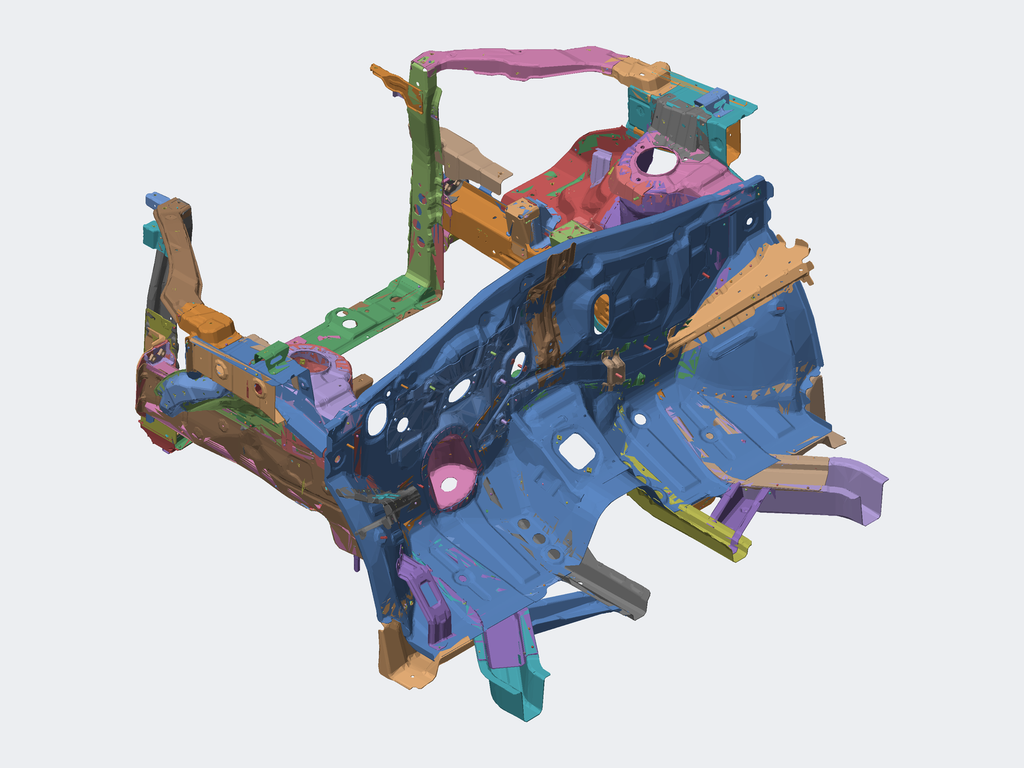Assembly | STEP file | 160 different items | 288 placed
Parts list (item | name | quantity | parent item):
1 | DAA9119051 | x2 | in FNA5301550
2 | FAN5301771 | x1 | in FNA5301770
3 | FNA5201125 | x9 | in FNA5301110, FNA5301240
4 | FNA5301010-H | x1 | in FNA5301010
5 | FNA5301020-H | x1 | in FNA5301020
6 | FNA5301030-H | x1 | in FNA5301030
7 | FNA5301040-H | x1 | in FNA5301040
8 | FNA5301051 | x1 | in FNA5301050
9 | FNA5301052 | x1 | in FNA5301060
10 | FNA5301100-H | x1 | in FNA5301100
11 | FNA5301101 | x1 | in FNA5301100
12 | FNA5301102 | x1 | in FNA5301100
13 | FNA5301103 | x1 | in FNA5301100
14 | FNA5301111 | x1 | in FNA5301110
15 | FNA5301120-H | x1 | in FNA5301120
16 | FNA5301121 | x2 | in FNA5301120
17 | FNA5301127 | x4 | in FNA5301110, FNA5301230, FNA5301750
18 | FNA5301131 | x1 | in FNA5301130
19 | FNA5301141 | x1 | in FNA5301140
20 | FNA5301151 | x1 | in FNA5301150
21 | FNA5301161 | x1 | in FNA5301160
22 | FNA5301171 | x1 | in FNA5301170
23 | FNA5301172 | x1 | in FNA5301180
24 | FNA5301191 | x1 | in FNA5301190
25 | FNA5301200-H | x1 | in FNA5301200
26 | FNA5301201 | x1 | in FNA5301200
27 | FNA5301202 | x1 | in FNA5301200
28 | FNA5301203 | x1 | in FNA5301980
29 | FNA5301204 | x1 | in FNA5301200
30 | FNA5301205 | x1 | in FNA5301020
31 | FNA5301211 | x1 | in FNA5301200
32 | FNA5301212 | x1 | in FNA5301220
33 | FNA5301231 | x1 | in FNA5301230
34 | FNA5301232 | x1 | in FNA5301240
35 | FNA5301252 | x1 | in FNA5301260
36 | FNA5301271 | x1 | in FNA5301270
37 | FNA5301272 | x1 | in FNA5301420
38 | FNA5301281 | x1 | in FNA5301280
39 | FNA5301291 | x1 | in FNA5301290
40 | FNA5301300-H | x1 | in FNA5301300
41 | FNA5301301 | x1 | in FNA5301030
42 | FNA5301302 | x1 | in FNA5301040
43 | FNA5301310-H | x1 | in FNA5301310
44 | FNA5301311 | x1 | in FNA5301310
45 | FNA5301312 | x1 | in FNA5301320
46 | FNA5301320-H | x1 | in FNA5301320
47 | FNA5301330-H | x1 | in FNA5301330
48 | FNA5301331 | x1 | in FNA5301410
49 | FNA5301332 | x1 | in FNA5301390
50 | FNA5301340-H | x1 | in FNA5301340
51 | FNA5301351 | x1 | in FNA5301350
52 | FNA5301352 | x1 | in FNA5301360
53 | FNA5301356 | x1 | in FNA5301380
54 | FNA5301400-H | x1 | in FNA5301400
55 | FNA5301410-H | x1 | in FNA5301410
56 | FNA5301420-H | x1 | in FNA5301420
57 | FNA5301430-H | x1 | in FNA5301430
58 | FNA5301431 | x1 | in FNA5301430
59 | FNA5301432 | x1 | in FNA5301440
60 | FNA5301440-H | x1 | in FNA5301440
61 | FNA5301451 | x1 | in FNA5301370
62 | FNA5301452 | x1 | in FNA5301460
63 | FNA5301453 | x1 | in FNA5301400
64 | FNA5301470-H | x1 | in FNA5301470
65 | FNA5301471 | x1 | in FNA5301470
66 | FNA5301472 | x1 | in FNA5301480
67 | FNA5301480-H | x1 | in FNA5301480
68 | FNA5301500-H | x1 | in FNA5301500
69 | FNA5301510-H | x1 | in FNA5301510
70 | FNA5301511 | x1 | in FNA5301510
71 | FNA5301512 | x1 | in FNA5301520
72 | FNA5301520-H | x1 | in FNA5301520
73 | FNA5301530-H | x1 | in FNA5301530
74 | FNA5301531 | x1 | in FNA5301530
75 | FNA5301532 | x1 | in FNA5301540
76 | FNA5301533 | x1 | in FNA5301530
77 | FNA5301534 | x1 | in FNA5301540
78 | FNA5301540-H | x1 | in FNA5301540
79 | FNA5301550-H | x1 | in FNA5301550
80 | FNA5301551 | x1 | in FNA5301550
81 | FNA5301552 | x1 | in FNA5301590
82 | FNA5301560-H | x1 | in FNA5301560
83 | FNA5301561 | x1 | in FNA5301560
84 | FNA5301562 | x1 | in FNA5301560
85 | FNA5301563 | x1 | in FNA5301560
86 | FNA5301571 | x1 | in FNA5301570
87 | FNA5301572 | x1 | in FNA5301580
88 | FNA5301600-H | x1 | in FNA5301600
89 | FNA5301611 | x1 | in FNA5301610
90 | FNA5301612 | x1 | in FNA5301620
91 | FNA5301630-H | x1 | in FNA5301630
92 | FNA5301631 | x1 | in FNA5301750
93 | FNA5301632 | x1 | in FNA5301760
94 | FNA5301651 | x1 | in FNA5301650
95 | FNA5301652 | x1 | in FNA5301630
96 | FNA5301661 | x1 | in FNA5301660
97 | FNA5301663 | x1 | in FNA5301910
98 | FNA5301664 | x1 | in FNA5301920
99 | FNA5301670-H | x1 | in FNA5301670
100 | FNA5301671 | x1 | in FNA5301670
101 | FNA5301672 | x1 | in FNA5301680
102 | FNA5301673 | x2 | in FNA5301670, FNA5301680
103 | FNA5301680-H | x1 | in FNA5301680
104 | FNA5301691 | x1 | in FNA5301690
105 | FNA5301711 | x1 | in FNA5301710
106 | FNA5301712 | x1 | in FNA5301720
107 | FNA5301731 | x1 | in FNA5301530
108 | FNA5301732 | x1 | in FNA5301540
109 | FNA5301750-H | x1 | in FNA5301750
110 | FNA5301760-H | x1 | in FNA5301760
111 | FNA5301772 | x1 | in FNA5301780
112 | FNA5301811 | x1 | in FNA5301810
113 | FNA5301820-H | x1 | in FNA5301820
114 | FNA5301821 | x2 | in FNA5301560, FNA5301820
115 | FNA5301831 | x1 | in FNA5301830
116 | FNA5301832 | x1 | in FNA5301840
117 | FNA5301833 | x1 | in FNA5301550
118 | FNA5301851 | x1 | in FNA5301850
119 | FNA5301871 | x1 | in FNA5301510
120 | FNA5301881 | x1 | in FNA5301880
121 | FNA5301891 | x1 | in FNA5301890
122 | FNA5301910-H | x1 | in FNA5301910
123 | FNA5301920-H | x1 | in FNA5301920
124 | FNA5301931 | x1 | in FNA5301930
125 | FNA5301932 | x1 | in FNA5301440
126 | FNA5301951 | x1 | in FNA5301950
127 | FNA5301952 | x1 | in FNA5301960
128 | FNA5301971 | x1 | in FNA5301510
129 | FNA8400020-H | x1 | in FNA8400020
130 | FNA8400200-H | x1 | in FNA8400200
131 | FNA8400201 | x1 | in FNA8400200
132 | FNA8400210-H | x1 | in FNA8400210
133 | FNA8400211 | x1 | in FNA8400290
134 | FNA8400212 | x1 | in FNA8400220
135 | FNA8400213 | x1 | in FNA8400210
136 | FNA8400214 | x1 | in FNA8400220
137 | FNA8400220-H | x1 | in FNA8400220
138 | FNA8400231 | x1 | in FNA8400230
139 | FNA8400232 | x1 | in FNA8400240
140 | FNA8400251 | x1 | in FNA8400250
141 | FNA8400261 | x1 | in FNA8400260
142 | FNA8400310-H | x1 | in FNA8400310
143 | FNA8400311 | x1 | in FNA8400310
144 | FNA8400312 | x1 | in FNA8400320
145 | FNA8400320-H | x1 | in FNA8400320
146 | FNA8400331 | x2 | in FNA8400330
147 | FNA8400361 | x1 | in FNA8400360
148 | FNA8400373 | x2 | in FNA8400370
149 | FNA8400411 | x1 | in FNA8400410
150 | FNA8400412 | x1 | in FNA8400420
151 | FNNA5301251 | x1 | in FNA5301250
152 | Q1100620 | x5 | in FNA5301110
153 | Q1980616 | x4 | in FNA5301150, FNA5301280, FNA5301980
154 | Q1980620 | x5 | in FNA5301150, FNA5301160, FNA5301220
155 | Q1980816 | x2 | in FNA5301150
156 | Q1980835 | x1 | in FNA5301590
157 | Q37106 | x70 | in FNA5301050, FNA5301060, FNA5301130, FNA5301140, FNA5301170, FNA5301180, FNA5301190, FNA5301250, FNA5301260, FNA5301270, FNA5301280, FNA5301350, FNA5301360, FNA5301370, FNA5301390, FNA5301460, FNA5301590, FNA5301770, FNA5301780, FNA5301810, FNA5301830, FNA5301840, FNA5301930, FNA5301950, FNA5301960, FNA8400250, FNA8400260, FNA8400290, FNA8400330, FNA8400360, FNA8400370, FNA8400410, FNA8400420
158 | Q37108 | x17 | in FNA5301260, FNA5301290, FNA5301380, FNA5301850, FNA5301880, FNA5301890, FNA8400230, FNA8400240, FNA8400360
159 | Q37110 | x14 | in FNA5301460, FNA5301570, FNA5301580, FNA5301610, FNA5301620, FNA5301650, FNA5301660, FNA5301690
160 | Q37114 | x2 | in FNA5301710, FNA5301720